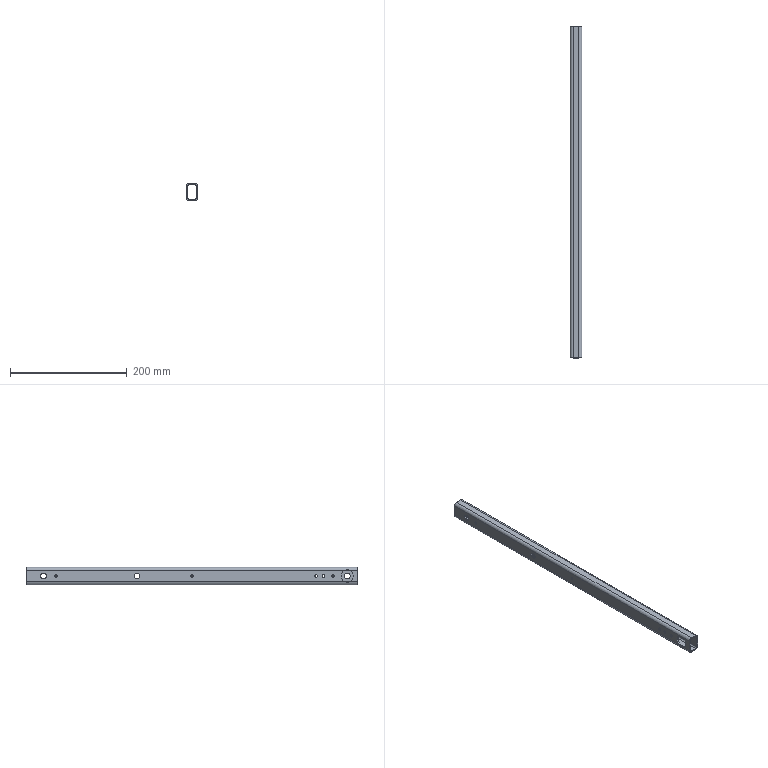Part | SolidWorks | features HoleWzd 2, ICE 1, WeldMemberFeat 1, WeldmentFeature 1 | 1 solid | 52 faces | box 20 x 568 x 30 mm | volume 116464 mm3 | cylinder 40 | plane 12 | commonest cylinder face diameters 4.2 x20 10 x14 5 x4 21 x2